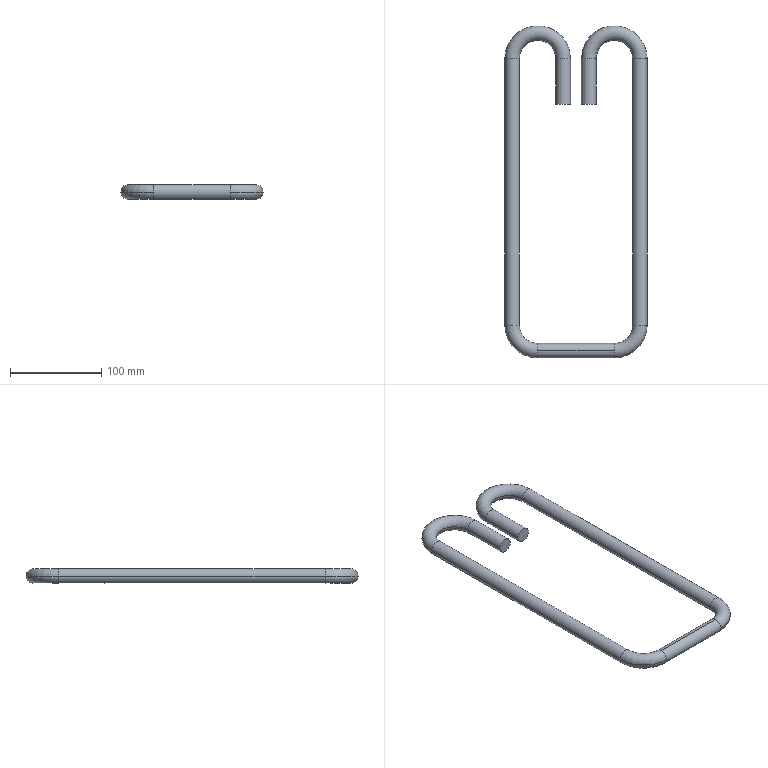Part | SolidWorks | features MirrorStock 1 | 1 solid | 20 faces | box 156 x 364 x 16 mm | volume 207475 mm3 | cylinder 10 | torus 8 | plane 2 | commonest cylinder face diameters 16 x10
STEP:
#1=CARTESIAN_POINT('',(6.,320.,0.));
#2=VERTEX_POINT('',#1);
#3=CARTESIAN_POINT('',(22.,320.,0.));
#4=VERTEX_POINT('',#3);
#5=CARTESIAN_POINT('',(14.,320.,0.));
#6=DIRECTION('',(0.,-1.,0.));
#7=DIRECTION('',(-1.,0.,0.));
#8=AXIS2_PLACEMENT_3D('',#5,#6,#7);
#9=CIRCLE('',#8,8.);
#10=EDGE_CURVE('',#2,#4,#9,.T.);
#11=ORIENTED_EDGE('',*,*,#10,.F.);
#12=CARTESIAN_POINT('',(78.,320.,0.));
#13=VERTEX_POINT('',#12);
#14=CARTESIAN_POINT('',(42.,320.,0.));
#15=DIRECTION('',(0.,0.,-1.));
#16=DIRECTION('',(0.,1.,0.));
#17=AXIS2_PLACEMENT_3D('',#14,#15,#16);
#18=CIRCLE('',#17,36.);
#19=EDGE_CURVE('',#2,#13,#18,.T.);
#20=ORIENTED_EDGE('',*,*,#19,.T.);
#21=CARTESIAN_POINT('',(62.,320.,0.));
#22=VERTEX_POINT('',#21);
#23=CARTESIAN_POINT('',(70.,320.,0.));
#24=DIRECTION('',(0.,1.,0.));
#25=DIRECTION('',(1.,0.,0.));
#26=AXIS2_PLACEMENT_3D('',#23,#24,#25);
#27=CIRCLE('',#26,8.);
#28=EDGE_CURVE('',#13,#22,#27,.T.);
#29=ORIENTED_EDGE('',*,*,#28,.T.);
#30=CARTESIAN_POINT('',(42.,320.,0.));
#31=DIRECTION('',(0.,0.,-1.));
#32=DIRECTION('',(0.,1.,0.));
#33=AXIS2_PLACEMENT_3D('',#30,#31,#32);
#34=CIRCLE('',#33,20.);
#35=EDGE_CURVE('',#4,#22,#34,.T.);
#36=ORIENTED_EDGE('',*,*,#35,.F.);
#37=EDGE_LOOP('',(#11,#20,#29,#36));
#38=FACE_OUTER_BOUND('',#37,.T.);
#39=CARTESIAN_POINT('',(42.,320.,0.));
#40=DIRECTION('',(0.,0.,-1.));
#41=DIRECTION('',(1.,0.,0.));
#42=AXIS2_PLACEMENT_3D('',#39,#40,#41);
#43=TOROIDAL_SURFACE('',#42,28.,8.);
#44=ADVANCED_FACE('',(#38),#43,.T.);
#45=CARTESIAN_POINT('',(78.,28.,0.));
#46=VERTEX_POINT('',#45);
#47=CARTESIAN_POINT('',(62.,28.,0.));
#48=VERTEX_POINT('',#47);
#49=CARTESIAN_POINT('',(70.,28.,0.));
#50=DIRECTION('',(0.,1.,0.));
#51=DIRECTION('',(1.,0.,0.));
#52=AXIS2_PLACEMENT_3D('',#49,#50,#51);
#53=CIRCLE('',#52,8.);
#54=EDGE_CURVE('',#46,#48,#53,.T.);
#55=ORIENTED_EDGE('',*,*,#54,.F.);
#56=CARTESIAN_POINT('',(42.,-8.,0.));
#57=VERTEX_POINT('',#56);
#58=CARTESIAN_POINT('',(42.,28.,0.));
#59=DIRECTION('',(0.,0.,-1.));
#60=DIRECTION('',(0.,1.,0.));
#61=AXIS2_PLACEMENT_3D('',#58,#59,#60);
#62=CIRCLE('',#61,36.);
#63=EDGE_CURVE('',#46,#57,#62,.T.);
#64=ORIENTED_EDGE('',*,*,#63,.T.);
#65=CARTESIAN_POINT('',(42.,0.,-8.));
#66=VERTEX_POINT('',#65);
#67=CARTESIAN_POINT('',(42.,0.,0.));
#68=DIRECTION('',(1.,0.,0.));
#69=DIRECTION('',(0.,-1.,0.));
#70=AXIS2_PLACEMENT_3D('',#67,#68,#69);
#71=CIRCLE('',#70,8.);
#72=EDGE_CURVE('',#57,#66,#71,.T.);
#73=ORIENTED_EDGE('',*,*,#72,.T.);
#74=CARTESIAN_POINT('',(42.,8.,0.));
#75=VERTEX_POINT('',#74);
#76=CARTESIAN_POINT('',(42.,0.,0.));
#77=DIRECTION('',(1.,0.,0.));
#78=DIRECTION('',(0.,-1.,0.));
#79=AXIS2_PLACEMENT_3D('',#76,#77,#78);
#80=CIRCLE('',#79,8.);
#81=EDGE_CURVE('',#66,#75,#80,.T.);
#82=ORIENTED_EDGE('',*,*,#81,.T.);
#83=CARTESIAN_POINT('',(42.,28.,0.));
#84=DIRECTION('',(0.,0.,-1.));
#85=DIRECTION('',(0.,1.,0.));
#86=AXIS2_PLACEMENT_3D('',#83,#84,#85);
#87=CIRCLE('',#86,20.);
#88=EDGE_CURVE('',#48,#75,#87,.T.);
#89=ORIENTED_EDGE('',*,*,#88,.F.);
#90=EDGE_LOOP('',(#55,#64,#73,#82,#89));
#91=FACE_OUTER_BOUND('',#90,.T.);
#92=CARTESIAN_POINT('',(42.,28.,0.));
#93=DIRECTION('',(0.,0.,-1.));
#94=DIRECTION('',(1.,0.,0.));
#95=AXIS2_PLACEMENT_3D('',#92,#93,#94);
#96=TOROIDAL_SURFACE('',#95,28.,8.);
#97=ADVANCED_FACE('',(#91),#96,.T.);
#98=CARTESIAN_POINT('',(-42.,-8.,0.));
#99=VERTEX_POINT('',#98);
#100=CARTESIAN_POINT('',(-42.,0.,-8.));
#101=VERTEX_POINT('',#100);
#102=CARTESIAN_POINT('',(-42.,0.,0.));
#103=DIRECTION('',(1.,0.,0.));
#104=DIRECTION('',(0.,-1.,0.));
#105=AXIS2_PLACEMENT_3D('',#102,#103,#104);
#106=CIRCLE('',#105,8.);
#107=EDGE_CURVE('',#99,#101,#106,.T.);
#108=ORIENTED_EDGE('',*,*,#107,.F.);
#109=CARTESIAN_POINT('',(-78.,28.,0.));
#110=VERTEX_POINT('',#109);
#111=CARTESIAN_POINT('',(-42.,28.,0.));
#112=DIRECTION('',(0.,0.,-1.));
#113=DIRECTION('',(0.,1.,0.));
#114=AXIS2_PLACEMENT_3D('',#111,#112,#113);
#115=CIRCLE('',#114,36.);
#116=EDGE_CURVE('',#99,#110,#115,.T.);
#117=ORIENTED_EDGE('',*,*,#116,.T.);
#118=CARTESIAN_POINT('',(-62.,28.,0.));
#119=VERTEX_POINT('',#118);
#120=CARTESIAN_POINT('',(-70.,28.,0.));
#121=DIRECTION('',(0.,-1.,0.));
#122=DIRECTION('',(-1.,0.,0.));
#123=AXIS2_PLACEMENT_3D('',#120,#121,#122);
#124=CIRCLE('',#123,8.);
#125=EDGE_CURVE('',#110,#119,#124,.T.);
#126=ORIENTED_EDGE('',*,*,#125,.T.);
#127=CARTESIAN_POINT('',(-42.,8.,0.));
#128=VERTEX_POINT('',#127);
#129=CARTESIAN_POINT('',(-42.,28.,0.));
#130=DIRECTION('',(0.,0.,-1.));
#131=DIRECTION('',(0.,1.,0.));
#132=AXIS2_PLACEMENT_3D('',#129,#130,#131);
#133=CIRCLE('',#132,20.);
#134=EDGE_CURVE('',#128,#119,#133,.T.);
#135=ORIENTED_EDGE('',*,*,#134,.F.);
#136=CARTESIAN_POINT('',(-42.,0.,0.));
#137=DIRECTION('',(1.,0.,0.));
#138=DIRECTION('',(0.,-1.,0.));
#139=AXIS2_PLACEMENT_3D('',#136,#137,#138);
#140=CIRCLE('',#139,8.);
#141=EDGE_CURVE('',#101,#128,#140,.T.);
#142=ORIENTED_EDGE('',*,*,#141,.F.);
#143=EDGE_LOOP('',(#108,#117,#126,#135,#142));
#144=FACE_OUTER_BOUND('',#143,.T.);
#145=CARTESIAN_POINT('',(-42.,28.,0.));
#146=DIRECTION('',(0.,0.,-1.));
#147=DIRECTION('',(1.,0.,0.));
#148=AXIS2_PLACEMENT_3D('',#145,#146,#147);
#149=TOROIDAL_SURFACE('',#148,28.,8.);
#150=ADVANCED_FACE('',(#144),#149,.T.);
#151=CARTESIAN_POINT('',(-78.,320.,0.));
#152=VERTEX_POINT('',#151);
#153=CARTESIAN_POINT('',(-62.,320.,0.));
#154=VERTEX_POINT('',#153);
#155=CARTESIAN_POINT('',(-70.,320.,0.));
#156=DIRECTION('',(0.,-1.,0.));
#157=DIRECTION('',(-1.,0.,0.));
#158=AXIS2_PLACEMENT_3D('',#155,#156,#157);
#159=CIRCLE('',#158,8.);
#160=EDGE_CURVE('',#152,#154,#159,.T.);
#161=ORIENTED_EDGE('',*,*,#160,.F.);
#162=CARTESIAN_POINT('',(-6.,320.,0.));
#163=VERTEX_POINT('',#162);
#164=CARTESIAN_POINT('',(-42.,320.,0.));
#165=DIRECTION('',(0.,0.,-1.));
#166=DIRECTION('',(0.,1.,0.));
#167=AXIS2_PLACEMENT_3D('',#164,#165,#166);
#168=CIRCLE('',#167,36.);
#169=EDGE_CURVE('',#152,#163,#168,.T.);
#170=ORIENTED_EDGE('',*,*,#169,.T.);
#171=CARTESIAN_POINT('',(-22.,320.,0.));
#172=VERTEX_POINT('',#171);
#173=CARTESIAN_POINT('',(-14.,320.,0.));
#174=DIRECTION('',(0.,1.,0.));
#175=DIRECTION('',(1.,0.,0.));
#176=AXIS2_PLACEMENT_3D('',#173,#174,#175);
#177=CIRCLE('',#176,8.);
#178=EDGE_CURVE('',#163,#172,#177,.T.);
#179=ORIENTED_EDGE('',*,*,#178,.T.);
#180=CARTESIAN_POINT('',(-42.,320.,0.));
#181=DIRECTION('',(0.,0.,-1.));
#182=DIRECTION('',(0.,1.,0.));
#183=AXIS2_PLACEMENT_3D('',#180,#181,#182);
#184=CIRCLE('',#183,20.);
#185=EDGE_CURVE('',#154,#172,#184,.T.);
#186=ORIENTED_EDGE('',*,*,#185,.F.);
#187=EDGE_LOOP('',(#161,#170,#179,#186));
#188=FACE_OUTER_BOUND('',#187,.T.);
#189=CARTESIAN_POINT('',(-42.,320.,0.));
#190=DIRECTION('',(0.,0.,-1.));
#191=DIRECTION('',(1.,0.,0.));
#192=AXIS2_PLACEMENT_3D('',#189,#190,#191);
#193=TOROIDAL_SURFACE('',#192,28.,8.);
#194=ADVANCED_FACE('',(#188),#193,.T.);
#195=CARTESIAN_POINT('',(14.,320.,0.));
#196=DIRECTION('',(0.,-1.,0.));
#197=DIRECTION('',(-1.,0.,0.));
#198=AXIS2_PLACEMENT_3D('',#195,#196,#197);
#199=CIRCLE('',#198,8.);
#200=EDGE_CURVE('',#4,#2,#199,.T.);
#201=ORIENTED_EDGE('',*,*,#200,.T.);
#202=CARTESIAN_POINT('',(6.,270.,0.));
#203=VERTEX_POINT('',#202);
#204=CARTESIAN_POINT('',(6.,320.,0.));
#205=DIRECTION('',(0.,-1.,0.));
#206=VECTOR('',#205,1000.);
#207=LINE('',#204,#206);
#208=EDGE_CURVE('',#2,#203,#207,.T.);
#209=ORIENTED_EDGE('',*,*,#208,.T.);
#210=CARTESIAN_POINT('',(22.,270.,0.));
#211=VERTEX_POINT('',#210);
#212=CARTESIAN_POINT('',(14.,270.,0.));
#213=DIRECTION('',(0.,-1.,0.));
#214=DIRECTION('',(-1.,0.,0.));
#215=AXIS2_PLACEMENT_3D('',#212,#213,#214);
#216=CIRCLE('',#215,8.);
#217=EDGE_CURVE('',#211,#203,#216,.T.);
#218=ORIENTED_EDGE('',*,*,#217,.F.);
#219=CARTESIAN_POINT('',(22.,320.,0.));
#220=DIRECTION('',(0.,-1.,0.));
#221=VECTOR('',#220,1000.);
#222=LINE('',#219,#221);
#223=EDGE_CURVE('',#4,#211,#222,.T.);
#224=ORIENTED_EDGE('',*,*,#223,.F.);
#225=EDGE_LOOP('',(#201,#209,#218,#224));
#226=FACE_OUTER_BOUND('',#225,.T.);
#227=CARTESIAN_POINT('',(14.,320.,0.));
#228=DIRECTION('',(0.,-1.,0.));
#229=DIRECTION('',(1.,0.,0.));
#230=AXIS2_PLACEMENT_3D('',#227,#228,#229);
#231=CYLINDRICAL_SURFACE('',#230,8.);
#232=ADVANCED_FACE('',(#226),#231,.T.);
#233=CARTESIAN_POINT('',(70.,28.,0.));
#234=DIRECTION('',(0.,1.,0.));
#235=DIRECTION('',(1.,0.,0.));
#236=AXIS2_PLACEMENT_3D('',#233,#234,#235);
#237=CIRCLE('',#236,8.);
#238=EDGE_CURVE('',#48,#46,#237,.T.);
#239=ORIENTED_EDGE('',*,*,#238,.T.);
#240=CARTESIAN_POINT('',(78.,28.,0.));
#241=DIRECTION('',(0.,1.,0.));
#242=VECTOR('',#241,1000.);
#243=LINE('',#240,#242);
#244=EDGE_CURVE('',#46,#13,#243,.T.);
#245=ORIENTED_EDGE('',*,*,#244,.T.);
#246=CARTESIAN_POINT('',(70.,320.,0.));
#247=DIRECTION('',(0.,1.,0.));
#248=DIRECTION('',(1.,0.,0.));
#249=AXIS2_PLACEMENT_3D('',#246,#247,#248);
#250=CIRCLE('',#249,8.);
#251=EDGE_CURVE('',#22,#13,#250,.T.);
#252=ORIENTED_EDGE('',*,*,#251,.F.);
#253=CARTESIAN_POINT('',(62.,28.,0.));
#254=DIRECTION('',(0.,1.,0.));
#255=VECTOR('',#254,1000.);
#256=LINE('',#253,#255);
#257=EDGE_CURVE('',#48,#22,#256,.T.);
#258=ORIENTED_EDGE('',*,*,#257,.F.);
#259=EDGE_LOOP('',(#239,#245,#252,#258));
#260=FACE_OUTER_BOUND('',#259,.T.);
#261=CARTESIAN_POINT('',(70.,28.,0.));
#262=DIRECTION('',(0.,1.,0.));
#263=DIRECTION('',(-1.,0.,0.));
#264=AXIS2_PLACEMENT_3D('',#261,#262,#263);
#265=CYLINDRICAL_SURFACE('',#264,8.);
#266=ADVANCED_FACE('',(#260),#265,.T.);
#267=CARTESIAN_POINT('',(-42.,0.,8.));
#268=VERTEX_POINT('',#267);
#269=CARTESIAN_POINT('',(-42.,0.,0.));
#270=DIRECTION('',(1.,0.,0.));
#271=DIRECTION('',(0.,-1.,0.));
#272=AXIS2_PLACEMENT_3D('',#269,#270,#271);
#273=CIRCLE('',#272,8.);
#274=EDGE_CURVE('',#268,#99,#273,.T.);
#275=ORIENTED_EDGE('',*,*,#274,.T.);
#276=ORIENTED_EDGE('',*,*,#107,.T.);
#277=CARTESIAN_POINT('',(-42.,0.,-8.));
#278=DIRECTION('',(1.,0.,0.));
#279=VECTOR('',#278,1000.);
#280=LINE('',#277,#279);
#281=EDGE_CURVE('',#101,#66,#280,.T.);
#282=ORIENTED_EDGE('',*,*,#281,.T.);
#283=ORIENTED_EDGE('',*,*,#72,.F.);
#284=CARTESIAN_POINT('',(42.,0.,8.));
#285=VERTEX_POINT('',#284);
#286=CARTESIAN_POINT('',(42.,0.,0.));
#287=DIRECTION('',(1.,0.,0.));
#288=DIRECTION('',(0.,-1.,0.));
#289=AXIS2_PLACEMENT_3D('',#286,#287,#288);
#290=CIRCLE('',#289,8.);
#291=EDGE_CURVE('',#285,#57,#290,.T.);
#292=ORIENTED_EDGE('',*,*,#291,.F.);
#293=CARTESIAN_POINT('',(-42.,0.,8.));
#294=DIRECTION('',(1.,0.,0.));
#295=VECTOR('',#294,1000.);
#296=LINE('',#293,#295);
#297=EDGE_CURVE('',#268,#285,#296,.T.);
#298=ORIENTED_EDGE('',*,*,#297,.F.);
#299=EDGE_LOOP('',(#275,#276,#282,#283,#292,#298));
#300=FACE_OUTER_BOUND('',#299,.T.);
#301=CARTESIAN_POINT('',(-42.,0.,0.));
#302=DIRECTION('',(1.,0.,0.));
#303=DIRECTION('',(0.,0.,1.));
#304=AXIS2_PLACEMENT_3D('',#301,#302,#303);
#305=CYLINDRICAL_SURFACE('',#304,8.);
#306=ADVANCED_FACE('',(#300),#305,.T.);
#307=CARTESIAN_POINT('',(-70.,320.,0.));
#308=DIRECTION('',(0.,-1.,0.));
#309=DIRECTION('',(-1.,0.,0.));
#310=AXIS2_PLACEMENT_3D('',#307,#308,#309);
#311=CIRCLE('',#310,8.);
#312=EDGE_CURVE('',#154,#152,#311,.T.);
#313=ORIENTED_EDGE('',*,*,#312,.T.);
#314=CARTESIAN_POINT('',(-78.,320.,0.));
#315=DIRECTION('',(0.,-1.,0.));
#316=VECTOR('',#315,1000.);
#317=LINE('',#314,#316);
#318=EDGE_CURVE('',#152,#110,#317,.T.);
#319=ORIENTED_EDGE('',*,*,#318,.T.);
#320=CARTESIAN_POINT('',(-70.,28.,0.));
#321=DIRECTION('',(0.,-1.,0.));
#322=DIRECTION('',(-1.,0.,0.));
#323=AXIS2_PLACEMENT_3D('',#320,#321,#322);
#324=CIRCLE('',#323,8.);
#325=EDGE_CURVE('',#119,#110,#324,.T.);
#326=ORIENTED_EDGE('',*,*,#325,.F.);
#327=CARTESIAN_POINT('',(-62.,320.,0.));
#328=DIRECTION('',(0.,-1.,0.));
#329=VECTOR('',#328,1000.);
#330=LINE('',#327,#329);
#331=EDGE_CURVE('',#154,#119,#330,.T.);
#332=ORIENTED_EDGE('',*,*,#331,.F.);
#333=EDGE_LOOP('',(#313,#319,#326,#332));
#334=FACE_OUTER_BOUND('',#333,.T.);
#335=CARTESIAN_POINT('',(-70.,320.,0.));
#336=DIRECTION('',(0.,-1.,0.));
#337=DIRECTION('',(1.,0.,0.));
#338=AXIS2_PLACEMENT_3D('',#335,#336,#337);
#339=CYLINDRICAL_SURFACE('',#338,8.);
#340=ADVANCED_FACE('',(#334),#339,.T.);
#341=CARTESIAN_POINT('',(-22.,270.,0.));
#342=VERTEX_POINT('',#341);
#343=CARTESIAN_POINT('',(-6.,270.,0.));
#344=VERTEX_POINT('',#343);
#345=CARTESIAN_POINT('',(-14.,270.,0.));
#346=DIRECTION('',(0.,1.,0.));
#347=DIRECTION('',(1.,0.,0.));
#348=AXIS2_PLACEMENT_3D('',#345,#346,#347);
#349=CIRCLE('',#348,8.);
#350=EDGE_CURVE('',#342,#344,#349,.T.);
#351=ORIENTED_EDGE('',*,*,#350,.T.);
#352=CARTESIAN_POINT('',(-6.,270.,0.));
#353=DIRECTION('',(0.,1.,0.));
#354=VECTOR('',#353,1000.);
#355=LINE('',#352,#354);
#356=EDGE_CURVE('',#344,#163,#355,.T.);
#357=ORIENTED_EDGE('',*,*,#356,.T.);
#358=CARTESIAN_POINT('',(-14.,320.,0.));
#359=DIRECTION('',(0.,1.,0.));
#360=DIRECTION('',(1.,0.,0.));
#361=AXIS2_PLACEMENT_3D('',#358,#359,#360);
#362=CIRCLE('',#361,8.);
#363=EDGE_CURVE('',#172,#163,#362,.T.);
#364=ORIENTED_EDGE('',*,*,#363,.F.);
#365=CARTESIAN_POINT('',(-22.,270.,0.));
#366=DIRECTION('',(0.,1.,0.));
#367=VECTOR('',#366,1000.);
#368=LINE('',#365,#367);
#369=EDGE_CURVE('',#342,#172,#368,.T.);
#370=ORIENTED_EDGE('',*,*,#369,.F.);
#371=EDGE_LOOP('',(#351,#357,#364,#370));
#372=FACE_OUTER_BOUND('',#371,.T.);
#373=CARTESIAN_POINT('',(-14.,270.,0.));
#374=DIRECTION('',(0.,1.,0.));
#375=DIRECTION('',(-1.,0.,0.));
#376=AXIS2_PLACEMENT_3D('',#373,#374,#375);
#377=CYLINDRICAL_SURFACE('',#376,8.);
#378=ADVANCED_FACE('',(#372),#377,.T.);
#379=ORIENTED_EDGE('',*,*,#350,.F.);
#380=CARTESIAN_POINT('',(-14.,270.,0.));
#381=DIRECTION('',(0.,1.,0.));
#382=DIRECTION('',(1.,0.,0.));
#383=AXIS2_PLACEMENT_3D('',#380,#381,#382);
#384=CIRCLE('',#383,8.);
#385=EDGE_CURVE('',#344,#342,#384,.T.);
#386=ORIENTED_EDGE('',*,*,#385,.F.);
#387=EDGE_LOOP('',(#379,#386));
#388=FACE_OUTER_BOUND('',#387,.T.);
#389=CARTESIAN_POINT('',(-14.,270.,0.));
#390=DIRECTION('',(0.,-1.,0.));
#391=DIRECTION('',(1.,0.,0.));
#392=AXIS2_PLACEMENT_3D('',#389,#390,#391);
#393=PLANE('',#392);
#394=ADVANCED_FACE('',(#388),#393,.T.);
#395=ORIENTED_EDGE('',*,*,#217,.T.);
#396=CARTESIAN_POINT('',(14.,270.,0.));
#397=DIRECTION('',(0.,-1.,0.));
#398=DIRECTION('',(-1.,0.,0.));
#399=AXIS2_PLACEMENT_3D('',#396,#397,#398);
#400=CIRCLE('',#399,8.);
#401=EDGE_CURVE('',#203,#211,#400,.T.);
#402=ORIENTED_EDGE('',*,*,#401,.T.);
#403=EDGE_LOOP('',(#395,#402));
#404=FACE_OUTER_BOUND('',#403,.T.);
#405=CARTESIAN_POINT('',(14.,270.,0.));
#406=DIRECTION('',(0.,1.,0.));
#407=DIRECTION('',(-1.,0.,0.));
#408=AXIS2_PLACEMENT_3D('',#405,#406,#407);
#409=PLANE('',#408);
#410=ADVANCED_FACE('',(#404),#409,.F.);
#411=ORIENTED_EDGE('',*,*,#356,.F.);
#412=ORIENTED_EDGE('',*,*,#385,.T.);
#413=ORIENTED_EDGE('',*,*,#369,.T.);
#414=ORIENTED_EDGE('',*,*,#178,.F.);
#415=EDGE_LOOP('',(#411,#412,#413,#414));
#416=FACE_OUTER_BOUND('',#415,.T.);
#417=CARTESIAN_POINT('',(-14.,270.,0.));
#418=DIRECTION('',(0.,1.,0.));
#419=DIRECTION('',(-1.,0.,0.));
#420=AXIS2_PLACEMENT_3D('',#417,#418,#419);
#421=CYLINDRICAL_SURFACE('',#420,8.);
#422=ADVANCED_FACE('',(#416),#421,.T.);
#423=ORIENTED_EDGE('',*,*,#169,.F.);
#424=ORIENTED_EDGE('',*,*,#312,.F.);
#425=ORIENTED_EDGE('',*,*,#185,.T.);
#426=ORIENTED_EDGE('',*,*,#363,.T.);
#427=EDGE_LOOP('',(#423,#424,#425,#426));
#428=FACE_OUTER_BOUND('',#427,.T.);
#429=CARTESIAN_POINT('',(-42.,320.,0.));
#430=DIRECTION('',(0.,0.,-1.));
#431=DIRECTION('',(1.,0.,0.));
#432=AXIS2_PLACEMENT_3D('',#429,#430,#431);
#433=TOROIDAL_SURFACE('',#432,28.,8.);
#434=ADVANCED_FACE('',(#428),#433,.T.);
#435=ORIENTED_EDGE('',*,*,#318,.F.);
#436=ORIENTED_EDGE('',*,*,#160,.T.);
#437=ORIENTED_EDGE('',*,*,#331,.T.);
#438=ORIENTED_EDGE('',*,*,#125,.F.);
#439=EDGE_LOOP('',(#435,#436,#437,#438));
#440=FACE_OUTER_BOUND('',#439,.T.);
#441=CARTESIAN_POINT('',(-70.,320.,0.));
#442=DIRECTION('',(0.,-1.,0.));
#443=DIRECTION('',(1.,0.,0.));
#444=AXIS2_PLACEMENT_3D('',#441,#442,#443);
#445=CYLINDRICAL_SURFACE('',#444,8.);
#446=ADVANCED_FACE('',(#440),#445,.T.);
#447=ORIENTED_EDGE('',*,*,#116,.F.);
#448=ORIENTED_EDGE('',*,*,#274,.F.);
#449=CARTESIAN_POINT('',(-42.,0.,0.));
#450=DIRECTION('',(1.,0.,0.));
#451=DIRECTION('',(0.,-1.,0.));
#452=AXIS2_PLACEMENT_3D('',#449,#450,#451);
#453=CIRCLE('',#452,8.);
#454=EDGE_CURVE('',#128,#268,#453,.T.);
#455=ORIENTED_EDGE('',*,*,#454,.F.);
#456=ORIENTED_EDGE('',*,*,#134,.T.);
#457=ORIENTED_EDGE('',*,*,#325,.T.);
#458=EDGE_LOOP('',(#447,#448,#455,#456,#457));
#459=FACE_OUTER_BOUND('',#458,.T.);
#460=CARTESIAN_POINT('',(-42.,28.,0.));
#461=DIRECTION('',(0.,0.,-1.));
#462=DIRECTION('',(1.,0.,0.));
#463=AXIS2_PLACEMENT_3D('',#460,#461,#462);
#464=TOROIDAL_SURFACE('',#463,28.,8.);
#465=ADVANCED_FACE('',(#459),#464,.T.);
#466=ORIENTED_EDGE('',*,*,#281,.F.);
#467=ORIENTED_EDGE('',*,*,#141,.T.);
#468=ORIENTED_EDGE('',*,*,#454,.T.);
#469=ORIENTED_EDGE('',*,*,#297,.T.);
#470=CARTESIAN_POINT('',(42.,0.,0.));
#471=DIRECTION('',(1.,0.,0.));
#472=DIRECTION('',(0.,-1.,0.));
#473=AXIS2_PLACEMENT_3D('',#470,#471,#472);
#474=CIRCLE('',#473,8.);
#475=EDGE_CURVE('',#75,#285,#474,.T.);
#476=ORIENTED_EDGE('',*,*,#475,.F.);
#477=ORIENTED_EDGE('',*,*,#81,.F.);
#478=EDGE_LOOP('',(#466,#467,#468,#469,#476,#477));
#479=FACE_OUTER_BOUND('',#478,.T.);
#480=CARTESIAN_POINT('',(-42.,0.,0.));
#481=DIRECTION('',(1.,0.,0.));
#482=DIRECTION('',(0.,0.,1.));
#483=AXIS2_PLACEMENT_3D('',#480,#481,#482);
#484=CYLINDRICAL_SURFACE('',#483,8.);
#485=ADVANCED_FACE('',(#479),#484,.T.);
#486=ORIENTED_EDGE('',*,*,#63,.F.);
#487=ORIENTED_EDGE('',*,*,#238,.F.);
#488=ORIENTED_EDGE('',*,*,#88,.T.);
#489=ORIENTED_EDGE('',*,*,#475,.T.);
#490=ORIENTED_EDGE('',*,*,#291,.T.);
#491=EDGE_LOOP('',(#486,#487,#488,#489,#490));
#492=FACE_OUTER_BOUND('',#491,.T.);
#493=CARTESIAN_POINT('',(42.,28.,0.));
#494=DIRECTION('',(0.,0.,-1.));
#495=DIRECTION('',(1.,0.,0.));
#496=AXIS2_PLACEMENT_3D('',#493,#494,#495);
#497=TOROIDAL_SURFACE('',#496,28.,8.);
#498=ADVANCED_FACE('',(#492),#497,.T.);
#499=ORIENTED_EDGE('',*,*,#244,.F.);
#500=ORIENTED_EDGE('',*,*,#54,.T.);
#501=ORIENTED_EDGE('',*,*,#257,.T.);
#502=ORIENTED_EDGE('',*,*,#28,.F.);
#503=EDGE_LOOP('',(#499,#500,#501,#502));
#504=FACE_OUTER_BOUND('',#503,.T.);
#505=CARTESIAN_POINT('',(70.,28.,0.));
#506=DIRECTION('',(0.,1.,0.));
#507=DIRECTION('',(-1.,0.,0.));
#508=AXIS2_PLACEMENT_3D('',#505,#506,#507);
#509=CYLINDRICAL_SURFACE('',#508,8.);
#510=ADVANCED_FACE('',(#504),#509,.T.);
#511=ORIENTED_EDGE('',*,*,#19,.F.);
#512=ORIENTED_EDGE('',*,*,#200,.F.);
#513=ORIENTED_EDGE('',*,*,#35,.T.);
#514=ORIENTED_EDGE('',*,*,#251,.T.);
#515=EDGE_LOOP('',(#511,#512,#513,#514));
#516=FACE_OUTER_BOUND('',#515,.T.);
#517=CARTESIAN_POINT('',(42.,320.,0.));
#518=DIRECTION('',(0.,0.,-1.));
#519=DIRECTION('',(1.,0.,0.));
#520=AXIS2_PLACEMENT_3D('',#517,#518,#519);
#521=TOROIDAL_SURFACE('',#520,28.,8.);
#522=ADVANCED_FACE('',(#516),#521,.T.);
#523=ORIENTED_EDGE('',*,*,#208,.F.);
#524=ORIENTED_EDGE('',*,*,#10,.T.);
#525=ORIENTED_EDGE('',*,*,#223,.T.);
#526=ORIENTED_EDGE('',*,*,#401,.F.);
#527=EDGE_LOOP('',(#523,#524,#525,#526));
#528=FACE_OUTER_BOUND('',#527,.T.);
#529=CARTESIAN_POINT('',(14.,320.,0.));
#530=DIRECTION('',(0.,-1.,0.));
#531=DIRECTION('',(1.,0.,0.));
#532=AXIS2_PLACEMENT_3D('',#529,#530,#531);
#533=CYLINDRICAL_SURFACE('',#532,8.);
#534=ADVANCED_FACE('',(#528),#533,.T.);
#535=CLOSED_SHELL('',(#44,#97,#150,#194,#232,#266,#306,#340,#378,#394,#410,#422,#434,#446,#465,#485,#498,#510,#522,#534));
#536=MANIFOLD_SOLID_BREP('',#535);
#537=CARTESIAN_POINT('',(0.,0.,0.));
#538=DIRECTION('',(0.,0.,1.));
#539=DIRECTION('',(1.,0.,0.));
#540=AXIS2_PLACEMENT_3D('',#537,#538,#539);
#541=(LENGTH_UNIT()NAMED_UNIT(*)SI_UNIT(.MILLI.,.METRE.));
#542=UNCERTAINTY_MEASURE_WITH_UNIT(LENGTH_MEASURE(0.00001),#541,'','');
#543=(NAMED_UNIT(*)PLANE_ANGLE_UNIT()SI_UNIT($,.RADIAN.));
#544=(NAMED_UNIT(*)SI_UNIT($,.STERADIAN.)SOLID_ANGLE_UNIT());
#545=(GEOMETRIC_REPRESENTATION_CONTEXT(3)GLOBAL_UNCERTAINTY_ASSIGNED_CONTEXT((#542))GLOBAL_UNIT_ASSIGNED_CONTEXT((#541,#543,#544))REPRESENTATION_CONTEXT('',''));
#546=ADVANCED_BREP_SHAPE_REPRESENTATION('',(#536,#540),#545);